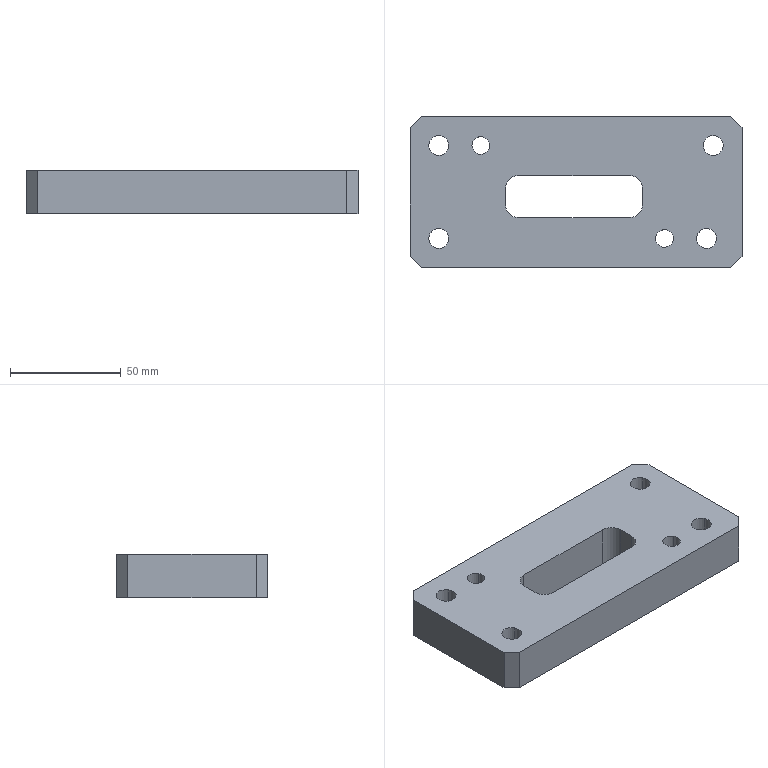Part | CATIA | 1 solid | 42 faces | box 150 x 68 x 19.5 mm | volume 164563 mm3 | cylinder 24 | plane 18 | commonest cylinder face diameters 9 x8 15 x8 8 x4 12 x4
STEP:
#1=CARTESIAN_POINT('',(-305.,34.,20.4));
#2=VERTEX_POINT('',#1);
#3=CARTESIAN_POINT('',(-300.,29.,20.4));
#4=VERTEX_POINT('',#3);
#5=CARTESIAN_POINT('',(-302.5,31.5,20.4));
#6=DIRECTION('',(-0.7071,0.7071,0.));
#7=VECTOR('',#6,1.);
#8=LINE('',#5,#7);
#9=EDGE_CURVE('',#2,#4,#8,.F.);
#10=ORIENTED_EDGE('',*,*,#9,.T.);
#11=CARTESIAN_POINT('',(-300.,29.,0.9));
#12=VERTEX_POINT('',#11);
#13=CARTESIAN_POINT('',(-300.,29.,10.65));
#14=DIRECTION('',(0.,0.,-1.));
#15=VECTOR('',#14,1.);
#16=LINE('',#13,#15);
#17=EDGE_CURVE('',#12,#4,#16,.F.);
#18=ORIENTED_EDGE('',*,*,#17,.F.);
#19=CARTESIAN_POINT('',(-305.,34.,0.9));
#20=VERTEX_POINT('',#19);
#21=CARTESIAN_POINT('',(-302.5,31.5,0.9));
#22=DIRECTION('',(-0.7071,0.7071,0.));
#23=VECTOR('',#22,1.);
#24=LINE('',#21,#23);
#25=EDGE_CURVE('',#12,#20,#24,.T.);
#26=ORIENTED_EDGE('',*,*,#25,.T.);
#27=CARTESIAN_POINT('',(-305.,34.,10.65));
#28=DIRECTION('',(0.,0.,-1.));
#29=VECTOR('',#28,1.);
#30=LINE('',#27,#29);
#31=EDGE_CURVE('',#20,#2,#30,.F.);
#32=ORIENTED_EDGE('',*,*,#31,.T.);
#33=EDGE_LOOP('',(#10,#18,#26,#32));
#34=FACE_OUTER_BOUND('',#33,.T.);
#35=CARTESIAN_POINT('',(-300.,29.,24.3));
#36=DIRECTION('',(0.7071,0.7071,0.));
#37=DIRECTION('',(0.,0.,-1.));
#38=AXIS2_PLACEMENT_3D('',#35,#36,#37);
#39=PLANE('',#38);
#40=ADVANCED_FACE('',(#34),#39,.T.);
#41=CARTESIAN_POINT('',(-445.,34.,0.9));
#42=VERTEX_POINT('',#41);
#43=CARTESIAN_POINT('',(-445.,34.,20.4));
#44=VERTEX_POINT('',#43);
#45=CARTESIAN_POINT('',(-445.,34.,10.65));
#46=DIRECTION('',(0.,0.,1.));
#47=VECTOR('',#46,1.);
#48=LINE('',#45,#47);
#49=EDGE_CURVE('',#42,#44,#48,.T.);
#50=ORIENTED_EDGE('',*,*,#49,.T.);
#51=CARTESIAN_POINT('',(-375.,34.,20.4));
#52=DIRECTION('',(1.,0.,0.));
#53=VECTOR('',#52,1.);
#54=LINE('',#51,#53);
#55=EDGE_CURVE('',#44,#2,#54,.T.);
#56=ORIENTED_EDGE('',*,*,#55,.T.);
#57=ORIENTED_EDGE('',*,*,#31,.F.);
#58=CARTESIAN_POINT('',(-375.,34.,0.9));
#59=DIRECTION('',(1.,0.,0.));
#60=VECTOR('',#59,1.);
#61=LINE('',#58,#60);
#62=EDGE_CURVE('',#20,#42,#61,.F.);
#63=ORIENTED_EDGE('',*,*,#62,.T.);
#64=EDGE_LOOP('',(#50,#56,#57,#63));
#65=FACE_OUTER_BOUND('',#64,.T.);
#66=CARTESIAN_POINT('',(-450.,34.,0.9));
#67=DIRECTION('',(0.,-1.,0.));
#68=DIRECTION('',(1.,0.,0.));
#69=AXIS2_PLACEMENT_3D('',#66,#67,#68);
#70=PLANE('',#69);
#71=ADVANCED_FACE('',(#65),#70,.F.);
#72=CARTESIAN_POINT('',(-450.,29.,20.4));
#73=VERTEX_POINT('',#72);
#74=CARTESIAN_POINT('',(-447.5,31.5,20.4));
#75=DIRECTION('',(0.7071,0.7071,0.));
#76=VECTOR('',#75,1.);
#77=LINE('',#74,#76);
#78=EDGE_CURVE('',#73,#44,#77,.T.);
#79=ORIENTED_EDGE('',*,*,#78,.T.);
#80=ORIENTED_EDGE('',*,*,#49,.F.);
#81=CARTESIAN_POINT('',(-450.,29.,0.9));
#82=VERTEX_POINT('',#81);
#83=CARTESIAN_POINT('',(-447.5,31.5,0.9));
#84=DIRECTION('',(0.7071,0.7071,0.));
#85=VECTOR('',#84,1.);
#86=LINE('',#83,#85);
#87=EDGE_CURVE('',#42,#82,#86,.F.);
#88=ORIENTED_EDGE('',*,*,#87,.T.);
#89=CARTESIAN_POINT('',(-450.,29.,10.65));
#90=DIRECTION('',(0.,0.,1.));
#91=VECTOR('',#90,1.);
#92=LINE('',#89,#91);
#93=EDGE_CURVE('',#82,#73,#92,.T.);
#94=ORIENTED_EDGE('',*,*,#93,.T.);
#95=EDGE_LOOP('',(#79,#80,#88,#94));
#96=FACE_OUTER_BOUND('',#95,.T.);
#97=CARTESIAN_POINT('',(-450.,29.,-3.));
#98=DIRECTION('',(-0.7071,0.7071,0.));
#99=DIRECTION('',(0.,0.,1.));
#100=AXIS2_PLACEMENT_3D('',#97,#98,#99);
#101=PLANE('',#100);
#102=ADVANCED_FACE('',(#96),#101,.T.);
#103=CARTESIAN_POINT('',(-450.,-29.,20.4));
#104=VERTEX_POINT('',#103);
#105=CARTESIAN_POINT('',(-450.,0.,20.4));
#106=DIRECTION('',(0.,-1.,0.));
#107=VECTOR('',#106,1.);
#108=LINE('',#105,#107);
#109=EDGE_CURVE('',#73,#104,#108,.T.);
#110=ORIENTED_EDGE('',*,*,#109,.F.);
#111=ORIENTED_EDGE('',*,*,#93,.F.);
#112=CARTESIAN_POINT('',(-450.,-29.,0.9));
#113=VERTEX_POINT('',#112);
#114=CARTESIAN_POINT('',(-450.,0.,0.9));
#115=DIRECTION('',(0.,-1.,0.));
#116=VECTOR('',#115,1.);
#117=LINE('',#114,#116);
#118=EDGE_CURVE('',#82,#113,#117,.T.);
#119=ORIENTED_EDGE('',*,*,#118,.T.);
#120=CARTESIAN_POINT('',(-450.,-29.,10.65));
#121=DIRECTION('',(0.,0.,-1.));
#122=VECTOR('',#121,1.);
#123=LINE('',#120,#122);
#124=EDGE_CURVE('',#113,#104,#123,.F.);
#125=ORIENTED_EDGE('',*,*,#124,.T.);
#126=EDGE_LOOP('',(#110,#111,#119,#125));
#127=FACE_OUTER_BOUND('',#126,.T.);
#128=CARTESIAN_POINT('',(-450.,34.,0.9));
#129=DIRECTION('',(-1.,0.,0.));
#130=DIRECTION('',(0.,-1.,0.));
#131=AXIS2_PLACEMENT_3D('',#128,#129,#130);
#132=PLANE('',#131);
#133=ADVANCED_FACE('',(#127),#132,.T.);
#134=CARTESIAN_POINT('',(-445.,-34.,20.4));
#135=VERTEX_POINT('',#134);
#136=CARTESIAN_POINT('',(-447.5,-31.5,20.4));
#137=DIRECTION('',(0.7071,-0.7071,0.));
#138=VECTOR('',#137,1.);
#139=LINE('',#136,#138);
#140=EDGE_CURVE('',#135,#104,#139,.F.);
#141=ORIENTED_EDGE('',*,*,#140,.T.);
#142=ORIENTED_EDGE('',*,*,#124,.F.);
#143=CARTESIAN_POINT('',(-445.,-34.,0.9));
#144=VERTEX_POINT('',#143);
#145=CARTESIAN_POINT('',(-447.5,-31.5,0.9));
#146=DIRECTION('',(0.7071,-0.7071,0.));
#147=VECTOR('',#146,1.);
#148=LINE('',#145,#147);
#149=EDGE_CURVE('',#113,#144,#148,.T.);
#150=ORIENTED_EDGE('',*,*,#149,.T.);
#151=CARTESIAN_POINT('',(-445.,-34.,10.65));
#152=DIRECTION('',(0.,0.,-1.));
#153=VECTOR('',#152,1.);
#154=LINE('',#151,#153);
#155=EDGE_CURVE('',#144,#135,#154,.F.);
#156=ORIENTED_EDGE('',*,*,#155,.T.);
#157=EDGE_LOOP('',(#141,#142,#150,#156));
#158=FACE_OUTER_BOUND('',#157,.T.);
#159=CARTESIAN_POINT('',(-450.,-29.,24.3));
#160=DIRECTION('',(-0.7071,-0.7071,0.));
#161=DIRECTION('',(0.,0.,-1.));
#162=AXIS2_PLACEMENT_3D('',#159,#160,#161);
#163=PLANE('',#162);
#164=ADVANCED_FACE('',(#158),#163,.T.);
#165=CARTESIAN_POINT('',(-300.,-29.,0.9));
#166=VERTEX_POINT('',#165);
#167=CARTESIAN_POINT('',(-300.,0.,0.9));
#168=DIRECTION('',(0.,1.,0.));
#169=VECTOR('',#168,1.);
#170=LINE('',#167,#169);
#171=EDGE_CURVE('',#166,#12,#170,.T.);
#172=ORIENTED_EDGE('',*,*,#171,.T.);
#173=ORIENTED_EDGE('',*,*,#17,.T.);
#174=CARTESIAN_POINT('',(-300.,-29.,20.4));
#175=VERTEX_POINT('',#174);
#176=CARTESIAN_POINT('',(-300.,0.,20.4));
#177=DIRECTION('',(0.,1.,0.));
#178=VECTOR('',#177,1.);
#179=LINE('',#176,#178);
#180=EDGE_CURVE('',#175,#4,#179,.T.);
#181=ORIENTED_EDGE('',*,*,#180,.F.);
#182=CARTESIAN_POINT('',(-300.,-29.,10.65));
#183=DIRECTION('',(0.,0.,1.));
#184=VECTOR('',#183,1.);
#185=LINE('',#182,#184);
#186=EDGE_CURVE('',#166,#175,#185,.T.);
#187=ORIENTED_EDGE('',*,*,#186,.F.);
#188=EDGE_LOOP('',(#172,#173,#181,#187));
#189=FACE_OUTER_BOUND('',#188,.T.);
#190=CARTESIAN_POINT('',(-300.,-34.,0.9));
#191=DIRECTION('',(1.,0.,0.));
#192=DIRECTION('',(0.,1.,0.));
#193=AXIS2_PLACEMENT_3D('',#190,#191,#192);
#194=PLANE('',#193);
#195=ADVANCED_FACE('',(#189),#194,.T.);
#196=CARTESIAN_POINT('',(-305.,-34.,0.9));
#197=VERTEX_POINT('',#196);
#198=CARTESIAN_POINT('',(-305.,-34.,20.4));
#199=VERTEX_POINT('',#198);
#200=CARTESIAN_POINT('',(-305.,-34.,10.65));
#201=DIRECTION('',(0.,0.,1.));
#202=VECTOR('',#201,1.);
#203=LINE('',#200,#202);
#204=EDGE_CURVE('',#197,#199,#203,.T.);
#205=ORIENTED_EDGE('',*,*,#204,.T.);
#206=CARTESIAN_POINT('',(-375.,-34.,20.4));
#207=DIRECTION('',(-1.,0.,0.));
#208=VECTOR('',#207,1.);
#209=LINE('',#206,#208);
#210=EDGE_CURVE('',#199,#135,#209,.T.);
#211=ORIENTED_EDGE('',*,*,#210,.T.);
#212=ORIENTED_EDGE('',*,*,#155,.F.);
#213=CARTESIAN_POINT('',(-375.,-34.,0.9));
#214=DIRECTION('',(-1.,0.,0.));
#215=VECTOR('',#214,1.);
#216=LINE('',#213,#215);
#217=EDGE_CURVE('',#144,#197,#216,.F.);
#218=ORIENTED_EDGE('',*,*,#217,.T.);
#219=EDGE_LOOP('',(#205,#211,#212,#218));
#220=FACE_OUTER_BOUND('',#219,.T.);
#221=CARTESIAN_POINT('',(-300.,-34.,0.9));
#222=DIRECTION('',(0.,1.,0.));
#223=DIRECTION('',(-1.,0.,0.));
#224=AXIS2_PLACEMENT_3D('',#221,#222,#223);
#225=PLANE('',#224);
#226=ADVANCED_FACE('',(#220),#225,.F.);
#227=CARTESIAN_POINT('',(-302.5,-31.5,20.4));
#228=DIRECTION('',(-0.7071,-0.7071,0.));
#229=VECTOR('',#228,1.);
#230=LINE('',#227,#229);
#231=EDGE_CURVE('',#175,#199,#230,.T.);
#232=ORIENTED_EDGE('',*,*,#231,.T.);
#233=ORIENTED_EDGE('',*,*,#204,.F.);
#234=CARTESIAN_POINT('',(-302.5,-31.5,0.9));
#235=DIRECTION('',(-0.7071,-0.7071,0.));
#236=VECTOR('',#235,1.);
#237=LINE('',#234,#236);
#238=EDGE_CURVE('',#197,#166,#237,.F.);
#239=ORIENTED_EDGE('',*,*,#238,.T.);
#240=ORIENTED_EDGE('',*,*,#186,.T.);
#241=EDGE_LOOP('',(#232,#233,#239,#240));
#242=FACE_OUTER_BOUND('',#241,.T.);
#243=CARTESIAN_POINT('',(-300.,-29.,-3.));
#244=DIRECTION('',(0.7071,-0.7071,0.));
#245=DIRECTION('',(0.,0.,1.));
#246=AXIS2_PLACEMENT_3D('',#243,#244,#245);
#247=PLANE('',#246);
#248=ADVANCED_FACE('',(#242),#247,.T.);
#249=CARTESIAN_POINT('',(-350.9,-11.6,20.4));
#250=VERTEX_POINT('',#249);
#251=CARTESIAN_POINT('',(-344.9,-5.6,20.4));
#252=VERTEX_POINT('',#251);
#253=CARTESIAN_POINT('',(-350.9,-5.6,20.4));
#254=DIRECTION('',(0.,0.,-1.));
#255=AXIS2_PLACEMENT_3D('',#253,#254,$);
#256=CIRCLE('',#255,6.);
#257=EDGE_CURVE('',#250,#252,#256,.F.);
#258=ORIENTED_EDGE('',*,*,#257,.T.);
#259=CARTESIAN_POINT('',(-344.9,-5.6,0.9));
#260=VERTEX_POINT('',#259);
#261=CARTESIAN_POINT('',(-344.9,-5.6,39.4));
#262=DIRECTION('',(0.,0.,-1.));
#263=VECTOR('',#262,1.);
#264=LINE('',#261,#263);
#265=EDGE_CURVE('',#252,#260,#264,.T.);
#266=ORIENTED_EDGE('',*,*,#265,.T.);
#267=CARTESIAN_POINT('',(-350.9,-11.6,0.9));
#268=VERTEX_POINT('',#267);
#269=CARTESIAN_POINT('',(-350.9,-5.6,0.9));
#270=DIRECTION('',(0.,0.,-1.));
#271=AXIS2_PLACEMENT_3D('',#269,#270,$);
#272=CIRCLE('',#271,6.);
#273=EDGE_CURVE('',#268,#260,#272,.F.);
#274=ORIENTED_EDGE('',*,*,#273,.F.);
#275=CARTESIAN_POINT('',(-350.9,-11.6,39.4));
#276=DIRECTION('',(0.,0.,-1.));
#277=VECTOR('',#276,1.);
#278=LINE('',#275,#277);
#279=EDGE_CURVE('',#250,#268,#278,.T.);
#280=ORIENTED_EDGE('',*,*,#279,.F.);
#281=EDGE_LOOP('',(#258,#266,#274,#280));
#282=FACE_OUTER_BOUND('',#281,.T.);
#283=CARTESIAN_POINT('',(-350.9,-5.6,39.4));
#284=DIRECTION('',(0.,0.,-1.));
#285=DIRECTION('',(1.,0.,0.));
#286=AXIS2_PLACEMENT_3D('',#283,#284,#285);
#287=CYLINDRICAL_SURFACE('',#286,6.);
#288=ADVANCED_FACE('',(#282),#287,.F.);
#289=ORIENTED_EDGE('',*,*,#279,.T.);
#290=CARTESIAN_POINT('',(-400.9,-11.6,0.9));
#291=VERTEX_POINT('',#290);
#292=CARTESIAN_POINT('',(-375.9,-11.6,0.9));
#293=DIRECTION('',(1.,0.,0.));
#294=VECTOR('',#293,1.);
#295=LINE('',#292,#294);
#296=EDGE_CURVE('',#291,#268,#295,.T.);
#297=ORIENTED_EDGE('',*,*,#296,.F.);
#298=CARTESIAN_POINT('',(-400.9,-11.6,20.4));
#299=VERTEX_POINT('',#298);
#300=CARTESIAN_POINT('',(-400.9,-11.6,39.4));
#301=DIRECTION('',(0.,0.,-1.));
#302=VECTOR('',#301,1.);
#303=LINE('',#300,#302);
#304=EDGE_CURVE('',#299,#291,#303,.T.);
#305=ORIENTED_EDGE('',*,*,#304,.F.);
#306=CARTESIAN_POINT('',(-375.9,-11.6,20.4));
#307=DIRECTION('',(1.,0.,0.));
#308=VECTOR('',#307,1.);
#309=LINE('',#306,#308);
#310=EDGE_CURVE('',#299,#250,#309,.T.);
#311=ORIENTED_EDGE('',*,*,#310,.T.);
#312=EDGE_LOOP('',(#289,#297,#305,#311));
#313=FACE_OUTER_BOUND('',#312,.T.);
#314=CARTESIAN_POINT('',(-401.9,-11.6,17.9));
#315=DIRECTION('',(0.,1.,0.));
#316=DIRECTION('',(1.,0.,0.));
#317=AXIS2_PLACEMENT_3D('',#314,#315,#316);
#318=PLANE('',#317);
#319=ADVANCED_FACE('',(#313),#318,.T.);
#320=CARTESIAN_POINT('',(-344.9,1.4,20.4));
#321=VERTEX_POINT('',#320);
#322=CARTESIAN_POINT('',(-344.9,-2.1,20.4));
#323=DIRECTION('',(0.,-1.,0.));
#324=VECTOR('',#323,1.);
#325=LINE('',#322,#324);
#326=EDGE_CURVE('',#321,#252,#325,.T.);
#327=ORIENTED_EDGE('',*,*,#326,.F.);
#328=CARTESIAN_POINT('',(-344.9,1.4,0.9));
#329=VERTEX_POINT('',#328);
#330=CARTESIAN_POINT('',(-344.9,1.4,39.4));
#331=DIRECTION('',(0.,0.,-1.));
#332=VECTOR('',#331,1.);
#333=LINE('',#330,#332);
#334=EDGE_CURVE('',#321,#329,#333,.T.);
#335=ORIENTED_EDGE('',*,*,#334,.T.);
#336=CARTESIAN_POINT('',(-344.9,-2.1,0.9));
#337=DIRECTION('',(0.,-1.,0.));
#338=VECTOR('',#337,1.);
#339=LINE('',#336,#338);
#340=EDGE_CURVE('',#260,#329,#339,.F.);
#341=ORIENTED_EDGE('',*,*,#340,.F.);
#342=ORIENTED_EDGE('',*,*,#265,.F.);
#343=EDGE_LOOP('',(#327,#335,#341,#342));
#344=FACE_OUTER_BOUND('',#343,.T.);
#345=CARTESIAN_POINT('',(-344.9,2.4,17.9));
#346=DIRECTION('',(1.,0.,0.));
#347=DIRECTION('',(0.,-1.,0.));
#348=AXIS2_PLACEMENT_3D('',#345,#346,#347);
#349=PLANE('',#348);
#350=ADVANCED_FACE('',(#344),#349,.F.);
#351=CARTESIAN_POINT('',(-406.9,-5.6,20.4));
#352=VERTEX_POINT('',#351);
#353=CARTESIAN_POINT('',(-400.9,-5.6,20.4));
#354=DIRECTION('',(0.,0.,-1.));
#355=AXIS2_PLACEMENT_3D('',#353,#354,$);
#356=CIRCLE('',#355,6.);
#357=EDGE_CURVE('',#352,#299,#356,.F.);
#358=ORIENTED_EDGE('',*,*,#357,.T.);
#359=ORIENTED_EDGE('',*,*,#304,.T.);
#360=CARTESIAN_POINT('',(-406.9,-5.6,0.9));
#361=VERTEX_POINT('',#360);
#362=CARTESIAN_POINT('',(-400.9,-5.6,0.9));
#363=DIRECTION('',(0.,0.,-1.));
#364=AXIS2_PLACEMENT_3D('',#362,#363,$);
#365=CIRCLE('',#364,6.);
#366=EDGE_CURVE('',#361,#291,#365,.F.);
#367=ORIENTED_EDGE('',*,*,#366,.F.);
#368=CARTESIAN_POINT('',(-406.9,-5.6,39.4));
#369=DIRECTION('',(0.,0.,-1.));
#370=VECTOR('',#369,1.);
#371=LINE('',#368,#370);
#372=EDGE_CURVE('',#352,#361,#371,.T.);
#373=ORIENTED_EDGE('',*,*,#372,.F.);
#374=EDGE_LOOP('',(#358,#359,#367,#373));
#375=FACE_OUTER_BOUND('',#374,.T.);
#376=CARTESIAN_POINT('',(-400.9,-5.6,39.4));
#377=DIRECTION('',(0.,0.,-1.));
#378=DIRECTION('',(0.,-1.,0.));
#379=AXIS2_PLACEMENT_3D('',#376,#377,#378);
#380=CYLINDRICAL_SURFACE('',#379,6.);
#381=ADVANCED_FACE('',(#375),#380,.F.);
#382=CARTESIAN_POINT('',(-350.9,7.4,20.4));
#383=VERTEX_POINT('',#382);
#384=CARTESIAN_POINT('',(-350.9,1.4,20.4));
#385=DIRECTION('',(0.,0.,-1.));
#386=AXIS2_PLACEMENT_3D('',#384,#385,$);
#387=CIRCLE('',#386,6.);
#388=EDGE_CURVE('',#321,#383,#387,.F.);
#389=ORIENTED_EDGE('',*,*,#388,.T.);
#390=CARTESIAN_POINT('',(-350.9,7.4,0.9));
#391=VERTEX_POINT('',#390);
#392=CARTESIAN_POINT('',(-350.9,7.4,39.4));
#393=DIRECTION('',(0.,0.,-1.));
#394=VECTOR('',#393,1.);
#395=LINE('',#392,#394);
#396=EDGE_CURVE('',#383,#391,#395,.T.);
#397=ORIENTED_EDGE('',*,*,#396,.T.);
#398=CARTESIAN_POINT('',(-350.9,1.4,0.9));
#399=DIRECTION('',(0.,0.,-1.));
#400=AXIS2_PLACEMENT_3D('',#398,#399,$);
#401=CIRCLE('',#400,6.);
#402=EDGE_CURVE('',#329,#391,#401,.F.);
#403=ORIENTED_EDGE('',*,*,#402,.F.);
#404=ORIENTED_EDGE('',*,*,#334,.F.);
#405=EDGE_LOOP('',(#389,#397,#403,#404));
#406=FACE_OUTER_BOUND('',#405,.T.);
#407=CARTESIAN_POINT('',(-350.9,1.4,39.4));
#408=DIRECTION('',(0.,0.,-1.));
#409=DIRECTION('',(0.,1.,0.));
#410=AXIS2_PLACEMENT_3D('',#407,#408,#409);
#411=CYLINDRICAL_SURFACE('',#410,6.);
#412=ADVANCED_FACE('',(#406),#411,.F.);
#413=CARTESIAN_POINT('',(-406.9,1.4,20.4));
#414=VERTEX_POINT('',#413);
#415=CARTESIAN_POINT('',(-406.9,-2.1,20.4));
#416=DIRECTION('',(0.,1.,0.));
#417=VECTOR('',#416,1.);
#418=LINE('',#415,#417);
#419=EDGE_CURVE('',#352,#414,#418,.T.);
#420=ORIENTED_EDGE('',*,*,#419,.F.);
#421=ORIENTED_EDGE('',*,*,#372,.T.);
#422=CARTESIAN_POINT('',(-406.9,1.4,0.9));
#423=VERTEX_POINT('',#422);
#424=CARTESIAN_POINT('',(-406.9,-2.1,0.9));
#425=DIRECTION('',(0.,1.,0.));
#426=VECTOR('',#425,1.);
#427=LINE('',#424,#426);
#428=EDGE_CURVE('',#361,#423,#427,.T.);
#429=ORIENTED_EDGE('',*,*,#428,.T.);
#430=CARTESIAN_POINT('',(-406.9,1.4,39.4));
#431=DIRECTION('',(0.,0.,-1.));
#432=VECTOR('',#431,1.);
#433=LINE('',#430,#432);
#434=EDGE_CURVE('',#414,#423,#433,.T.);
#435=ORIENTED_EDGE('',*,*,#434,.F.);
#436=EDGE_LOOP('',(#420,#421,#429,#435));
#437=FACE_OUTER_BOUND('',#436,.T.);
#438=CARTESIAN_POINT('',(-406.9,-6.6,17.9));
#439=DIRECTION('',(-1.,0.,0.));
#440=DIRECTION('',(0.,1.,0.));
#441=AXIS2_PLACEMENT_3D('',#438,#439,#440);
#442=PLANE('',#441);
#443=ADVANCED_FACE('',(#437),#442,.F.);
#444=CARTESIAN_POINT('',(-400.9,7.4,20.4));
#445=VERTEX_POINT('',#444);
#446=CARTESIAN_POINT('',(-400.9,7.4,0.9));
#447=VERTEX_POINT('',#446);
#448=CARTESIAN_POINT('',(-400.9,7.4,39.4));
#449=DIRECTION('',(0.,0.,-1.));
#450=VECTOR('',#449,1.);
#451=LINE('',#448,#450);
#452=EDGE_CURVE('',#445,#447,#451,.T.);
#453=ORIENTED_EDGE('',*,*,#452,.T.);
#454=CARTESIAN_POINT('',(-375.9,7.4,0.9));
#455=DIRECTION('',(-1.,0.,0.));
#456=VECTOR('',#455,1.);
#457=LINE('',#454,#456);
#458=EDGE_CURVE('',#447,#391,#457,.F.);
#459=ORIENTED_EDGE('',*,*,#458,.T.);
#460=ORIENTED_EDGE('',*,*,#396,.F.);
#461=CARTESIAN_POINT('',(-375.9,7.4,20.4));
#462=DIRECTION('',(-1.,0.,0.));
#463=VECTOR('',#462,1.);
#464=LINE('',#461,#463);
#465=EDGE_CURVE('',#383,#445,#464,.T.);
#466=ORIENTED_EDGE('',*,*,#465,.T.);
#467=EDGE_LOOP('',(#453,#459,#460,#466));
#468=FACE_OUTER_BOUND('',#467,.T.);
#469=CARTESIAN_POINT('',(-349.9,7.4,17.9));
#470=DIRECTION('',(0.,-1.,0.));
#471=DIRECTION('',(-1.,0.,0.));
#472=AXIS2_PLACEMENT_3D('',#469,#470,#471);
#473=PLANE('',#472);
#474=ADVANCED_FACE('',(#468),#473,.T.);
#475=CARTESIAN_POINT('',(-400.9,1.4,20.4));
#476=DIRECTION('',(0.,0.,-1.));
#477=AXIS2_PLACEMENT_3D('',#475,#476,$);
#478=CIRCLE('',#477,6.);
#479=EDGE_CURVE('',#445,#414,#478,.F.);
#480=ORIENTED_EDGE('',*,*,#479,.T.);
#481=ORIENTED_EDGE('',*,*,#434,.T.);
#482=CARTESIAN_POINT('',(-400.9,1.4,0.9));
#483=DIRECTION('',(0.,0.,-1.));
#484=AXIS2_PLACEMENT_3D('',#482,#483,$);
#485=CIRCLE('',#484,6.);
#486=EDGE_CURVE('',#447,#423,#485,.F.);
#487=ORIENTED_EDGE('',*,*,#486,.F.);
#488=ORIENTED_EDGE('',*,*,#452,.F.);
#489=EDGE_LOOP('',(#480,#481,#487,#488));
#490=FACE_OUTER_BOUND('',#489,.T.);
#491=CARTESIAN_POINT('',(-400.9,1.4,39.4));
#492=DIRECTION('',(0.,0.,-1.));
#493=DIRECTION('',(-1.,0.,0.));
#494=AXIS2_PLACEMENT_3D('',#491,#492,#493);
#495=CYLINDRICAL_SURFACE('',#494,6.);
#496=ADVANCED_FACE('',(#490),#495,.F.);
#497=ORIENTED_EDGE('',*,*,#238,.F.);
#498=ORIENTED_EDGE('',*,*,#217,.F.);
#499=ORIENTED_EDGE('',*,*,#149,.F.);
#500=ORIENTED_EDGE('',*,*,#118,.F.);
#501=ORIENTED_EDGE('',*,*,#87,.F.);
#502=ORIENTED_EDGE('',*,*,#62,.F.);
#503=ORIENTED_EDGE('',*,*,#25,.F.);
#504=ORIENTED_EDGE('',*,*,#171,.F.);
#505=EDGE_LOOP('',(#497,#498,#499,#500,#501,#502,#503,#504));
#506=FACE_OUTER_BOUND('',#505,.T.);
#507=ORIENTED_EDGE('',*,*,#273,.T.);
#508=ORIENTED_EDGE('',*,*,#340,.T.);
#509=ORIENTED_EDGE('',*,*,#402,.T.);
#510=ORIENTED_EDGE('',*,*,#458,.F.);
#511=ORIENTED_EDGE('',*,*,#486,.T.);
#512=ORIENTED_EDGE('',*,*,#428,.F.);
#513=ORIENTED_EDGE('',*,*,#366,.T.);
#514=ORIENTED_EDGE('',*,*,#296,.T.);
#515=EDGE_LOOP('',(#507,#508,#509,#510,#511,#512,#513,#514));
#516=FACE_BOUND('',#515,.T.);
#517=CARTESIAN_POINT('',(-306.418,24.596,0.9));
#518=VERTEX_POINT('',#517);
#519=CARTESIAN_POINT('',(-319.582,17.404,0.9));
#520=VERTEX_POINT('',#519);
#521=CARTESIAN_POINT('',(-313.,21.,0.9));
#522=DIRECTION('',(0.,0.,1.));
#523=AXIS2_PLACEMENT_3D('',#521,#522,$);
#524=CIRCLE('',#523,7.5);
#525=EDGE_CURVE('',#518,#520,#524,.T.);
#526=ORIENTED_EDGE('',*,*,#525,.T.);
#527=CARTESIAN_POINT('',(-313.,21.,0.9));
#528=DIRECTION('',(0.,0.,1.));
#529=AXIS2_PLACEMENT_3D('',#527,#528,$);
#530=CIRCLE('',#529,7.5);
#531=EDGE_CURVE('',#520,#518,#530,.T.);
#532=ORIENTED_EDGE('',*,*,#531,.T.);
#533=EDGE_LOOP('',(#526,#532));
#534=FACE_BOUND('',#533,.T.);
#535=CARTESIAN_POINT('',(-430.418,24.596,0.9));
#536=VERTEX_POINT('',#535);
#537=CARTESIAN_POINT('',(-443.582,17.404,0.9));
#538=VERTEX_POINT('',#537);
#539=CARTESIAN_POINT('',(-437.,21.,0.9));
#540=DIRECTION('',(0.,0.,1.));
#541=AXIS2_PLACEMENT_3D('',#539,#540,$);
#542=CIRCLE('',#541,7.5);
#543=EDGE_CURVE('',#536,#538,#542,.T.);
#544=ORIENTED_EDGE('',*,*,#543,.T.);
#545=CARTESIAN_POINT('',(-437.,21.,0.9));
#546=DIRECTION('',(0.,0.,1.));
#547=AXIS2_PLACEMENT_3D('',#545,#546,$);
#548=CIRCLE('',#547,7.5);
#549=EDGE_CURVE('',#538,#536,#548,.T.);
#550=ORIENTED_EDGE('',*,*,#549,.T.);
#551=EDGE_LOOP('',(#544,#550));
#552=FACE_BOUND('',#551,.T.);
#553=CARTESIAN_POINT('',(-430.418,-17.404,0.9));
#554=VERTEX_POINT('',#553);
#555=CARTESIAN_POINT('',(-443.582,-24.596,0.9));
#556=VERTEX_POINT('',#555);
#557=CARTESIAN_POINT('',(-437.,-21.,0.9));
#558=DIRECTION('',(0.,0.,1.));
#559=AXIS2_PLACEMENT_3D('',#557,#558,$);
#560=CIRCLE('',#559,7.5);
#561=EDGE_CURVE('',#554,#556,#560,.T.);
#562=ORIENTED_EDGE('',*,*,#561,.T.);
#563=CARTESIAN_POINT('',(-437.,-21.,0.9));
#564=DIRECTION('',(0.,0.,1.));
#565=AXIS2_PLACEMENT_3D('',#563,#564,$);
#566=CIRCLE('',#565,7.5);
#567=EDGE_CURVE('',#556,#554,#566,.T.);
#568=ORIENTED_EDGE('',*,*,#567,.T.);
#569=EDGE_LOOP('',(#562,#568));
#570=FACE_BOUND('',#569,.T.);
#571=CARTESIAN_POINT('',(-309.418,-17.404,0.9));
#572=VERTEX_POINT('',#571);
#573=CARTESIAN_POINT('',(-322.582,-24.596,0.9));
#574=VERTEX_POINT('',#573);
#575=CARTESIAN_POINT('',(-316.,-21.,0.9));
#576=DIRECTION('',(0.,0.,1.));
#577=AXIS2_PLACEMENT_3D('',#575,#576,$);
#578=CIRCLE('',#577,7.5);
#579=EDGE_CURVE('',#572,#574,#578,.T.);
#580=ORIENTED_EDGE('',*,*,#579,.T.);
#581=CARTESIAN_POINT('',(-316.,-21.,0.9));
#582=DIRECTION('',(0.,0.,1.));
#583=AXIS2_PLACEMENT_3D('',#581,#582,$);
#584=CIRCLE('',#583,7.5);
#585=EDGE_CURVE('',#574,#572,#584,.T.);
#586=ORIENTED_EDGE('',*,*,#585,.T.);
#587=EDGE_LOOP('',(#580,#586));
#588=FACE_BOUND('',#587,.T.);
#589=CARTESIAN_POINT('',(-338.51,-22.918,0.9));
#590=VERTEX_POINT('',#589);
#591=CARTESIAN_POINT('',(-331.49,-19.082,0.9));
#592=VERTEX_POINT('',#591);
#593=CARTESIAN_POINT('',(-335.,-21.,0.9));
#594=DIRECTION('',(0.,0.,1.));
#595=AXIS2_PLACEMENT_3D('',#593,#594,$);
#596=CIRCLE('',#595,4.);
#597=EDGE_CURVE('',#590,#592,#596,.T.);
#598=ORIENTED_EDGE('',*,*,#597,.T.);
#599=CARTESIAN_POINT('',(-335.,-21.,0.9));
#600=DIRECTION('',(0.,0.,1.));
#601=AXIS2_PLACEMENT_3D('',#599,#600,$);
#602=CIRCLE('',#601,4.);
#603=EDGE_CURVE('',#592,#590,#602,.T.);
#604=ORIENTED_EDGE('',*,*,#603,.T.);
#605=EDGE_LOOP('',(#598,#604));
#606=FACE_BOUND('',#605,.T.);
#607=CARTESIAN_POINT('',(-421.51,19.082,0.9));
#608=VERTEX_POINT('',#607);
#609=CARTESIAN_POINT('',(-414.49,22.918,0.9));
#610=VERTEX_POINT('',#609);
#611=CARTESIAN_POINT('',(-418.,21.,0.9));
#612=DIRECTION('',(0.,0.,1.));
#613=AXIS2_PLACEMENT_3D('',#611,#612,$);
#614=CIRCLE('',#613,4.);
#615=EDGE_CURVE('',#608,#610,#614,.T.);
#616=ORIENTED_EDGE('',*,*,#615,.T.);
#617=CARTESIAN_POINT('',(-418.,21.,0.9));
#618=DIRECTION('',(0.,0.,1.));
#619=AXIS2_PLACEMENT_3D('',#617,#618,$);
#620=CIRCLE('',#619,4.);
#621=EDGE_CURVE('',#610,#608,#620,.T.);
#622=ORIENTED_EDGE('',*,*,#621,.T.);
#623=EDGE_LOOP('',(#616,#622));
#624=FACE_BOUND('',#623,.T.);
#625=CARTESIAN_POINT('',(0.,0.,0.9));
#626=DIRECTION('',(0.,0.,1.));
#627=DIRECTION('',(1.,0.,0.));
#628=AXIS2_PLACEMENT_3D('',#625,#626,#627);
#629=PLANE('',#628);
#630=ADVANCED_FACE('',(#506,#516,#534,#552,#570,#588,#606,#624),#629,.F.);
#631=ORIENTED_EDGE('',*,*,#180,.T.);
#632=ORIENTED_EDGE('',*,*,#9,.F.);
#633=ORIENTED_EDGE('',*,*,#55,.F.);
#634=ORIENTED_EDGE('',*,*,#78,.F.);
#635=ORIENTED_EDGE('',*,*,#109,.T.);
#636=ORIENTED_EDGE('',*,*,#140,.F.);
#637=ORIENTED_EDGE('',*,*,#210,.F.);
#638=ORIENTED_EDGE('',*,*,#231,.F.);
#639=EDGE_LOOP('',(#631,#632,#633,#634,#635,#636,#637,#638));
#640=FACE_OUTER_BOUND('',#639,.T.);
#641=ORIENTED_EDGE('',*,*,#310,.F.);
#642=ORIENTED_EDGE('',*,*,#357,.F.);
#643=ORIENTED_EDGE('',*,*,#419,.T.);
#644=ORIENTED_EDGE('',*,*,#479,.F.);
#645=ORIENTED_EDGE('',*,*,#465,.F.);
#646=ORIENTED_EDGE('',*,*,#388,.F.);
#647=ORIENTED_EDGE('',*,*,#326,.T.);
#648=ORIENTED_EDGE('',*,*,#257,.F.);
#649=EDGE_LOOP('',(#641,#642,#643,#644,#645,#646,#647,#648));
#650=FACE_BOUND('',#649,.T.);
#651=CARTESIAN_POINT('',(-316.949,18.843,20.4));
#652=VERTEX_POINT('',#651);
#653=CARTESIAN_POINT('',(-309.051,23.157,20.4));
#654=VERTEX_POINT('',#653);
#655=CARTESIAN_POINT('',(-313.,21.,20.4));
#656=DIRECTION('',(0.,0.,1.));
#657=AXIS2_PLACEMENT_3D('',#655,#656,$);
#658=CIRCLE('',#657,4.5);
#659=EDGE_CURVE('',#652,#654,#658,.T.);
#660=ORIENTED_EDGE('',*,*,#659,.F.);
#661=CARTESIAN_POINT('',(-313.,21.,20.4));
#662=DIRECTION('',(0.,0.,1.));
#663=AXIS2_PLACEMENT_3D('',#661,#662,$);
#664=CIRCLE('',#663,4.5);
#665=EDGE_CURVE('',#654,#652,#664,.T.);
#666=ORIENTED_EDGE('',*,*,#665,.F.);
#667=EDGE_LOOP('',(#660,#666));
#668=FACE_BOUND('',#667,.T.);
#669=CARTESIAN_POINT('',(-440.949,18.843,20.4));
#670=VERTEX_POINT('',#669);
#671=CARTESIAN_POINT('',(-433.051,23.157,20.4));
#672=VERTEX_POINT('',#671);
#673=CARTESIAN_POINT('',(-437.,21.,20.4));
#674=DIRECTION('',(0.,0.,1.));
#675=AXIS2_PLACEMENT_3D('',#673,#674,$);
#676=CIRCLE('',#675,4.5);
#677=EDGE_CURVE('',#670,#672,#676,.T.);
#678=ORIENTED_EDGE('',*,*,#677,.F.);
#679=CARTESIAN_POINT('',(-437.,21.,20.4));
#680=DIRECTION('',(0.,0.,1.));
#681=AXIS2_PLACEMENT_3D('',#679,#680,$);
#682=CIRCLE('',#681,4.5);
#683=EDGE_CURVE('',#672,#670,#682,.T.);
#684=ORIENTED_EDGE('',*,*,#683,.F.);
#685=EDGE_LOOP('',(#678,#684));
#686=FACE_BOUND('',#685,.T.);
#687=CARTESIAN_POINT('',(-440.949,-23.157,20.4));
#688=VERTEX_POINT('',#687);
#689=CARTESIAN_POINT('',(-433.051,-18.843,20.4));
#690=VERTEX_POINT('',#689);
#691=CARTESIAN_POINT('',(-437.,-21.,20.4));
#692=DIRECTION('',(0.,0.,1.));
#693=AXIS2_PLACEMENT_3D('',#691,#692,$);
#694=CIRCLE('',#693,4.5);
#695=EDGE_CURVE('',#688,#690,#694,.T.);
#696=ORIENTED_EDGE('',*,*,#695,.F.);
#697=CARTESIAN_POINT('',(-437.,-21.,20.4));
#698=DIRECTION('',(0.,0.,1.));
#699=AXIS2_PLACEMENT_3D('',#697,#698,$);
#700=CIRCLE('',#699,4.5);
#701=EDGE_CURVE('',#690,#688,#700,.T.);
#702=ORIENTED_EDGE('',*,*,#701,.F.);
#703=EDGE_LOOP('',(#696,#702));
#704=FACE_BOUND('',#703,.T.);
#705=CARTESIAN_POINT('',(-319.949,-23.157,20.4));
#706=VERTEX_POINT('',#705);
#707=CARTESIAN_POINT('',(-312.051,-18.843,20.4));
#708=VERTEX_POINT('',#707);
#709=CARTESIAN_POINT('',(-316.,-21.,20.4));
#710=DIRECTION('',(0.,0.,1.));
#711=AXIS2_PLACEMENT_3D('',#709,#710,$);
#712=CIRCLE('',#711,4.5);
#713=EDGE_CURVE('',#706,#708,#712,.T.);
#714=ORIENTED_EDGE('',*,*,#713,.F.);
#715=CARTESIAN_POINT('',(-316.,-21.,20.4));
#716=DIRECTION('',(0.,0.,1.));
#717=AXIS2_PLACEMENT_3D('',#715,#716,$);
#718=CIRCLE('',#717,4.5);
#719=EDGE_CURVE('',#708,#706,#718,.T.);
#720=ORIENTED_EDGE('',*,*,#719,.F.);
#721=EDGE_LOOP('',(#714,#720));
#722=FACE_BOUND('',#721,.T.);
#723=CARTESIAN_POINT('',(-338.51,-22.918,20.4));
#724=VERTEX_POINT('',#723);
#725=CARTESIAN_POINT('',(-331.49,-19.082,20.4));
#726=VERTEX_POINT('',#725);
#727=CARTESIAN_POINT('',(-335.,-21.,20.4));
#728=DIRECTION('',(0.,0.,1.));
#729=AXIS2_PLACEMENT_3D('',#727,#728,$);
#730=CIRCLE('',#729,4.);
#731=EDGE_CURVE('',#724,#726,#730,.T.);
#732=ORIENTED_EDGE('',*,*,#731,.F.);
#733=CARTESIAN_POINT('',(-335.,-21.,20.4));
#734=DIRECTION('',(0.,0.,1.));
#735=AXIS2_PLACEMENT_3D('',#733,#734,$);
#736=CIRCLE('',#735,4.);
#737=EDGE_CURVE('',#726,#724,#736,.T.);
#738=ORIENTED_EDGE('',*,*,#737,.F.);
#739=EDGE_LOOP('',(#732,#738));
#740=FACE_BOUND('',#739,.T.);
#741=CARTESIAN_POINT('',(-421.51,19.082,20.4));
#742=VERTEX_POINT('',#741);
#743=CARTESIAN_POINT('',(-414.49,22.918,20.4));
#744=VERTEX_POINT('',#743);
#745=CARTESIAN_POINT('',(-418.,21.,20.4));
#746=DIRECTION('',(0.,0.,1.));
#747=AXIS2_PLACEMENT_3D('',#745,#746,$);
#748=CIRCLE('',#747,4.);
#749=EDGE_CURVE('',#742,#744,#748,.T.);
#750=ORIENTED_EDGE('',*,*,#749,.F.);
#751=CARTESIAN_POINT('',(-418.,21.,20.4));
#752=DIRECTION('',(0.,0.,1.));
#753=AXIS2_PLACEMENT_3D('',#751,#752,$);
#754=CIRCLE('',#753,4.);
#755=EDGE_CURVE('',#744,#742,#754,.T.);
#756=ORIENTED_EDGE('',*,*,#755,.F.);
#757=EDGE_LOOP('',(#750,#756));
#758=FACE_BOUND('',#757,.T.);
#759=CARTESIAN_POINT('',(0.,0.,20.4));
#760=DIRECTION('',(0.,0.,1.));
#761=DIRECTION('',(1.,0.,0.));
#762=AXIS2_PLACEMENT_3D('',#759,#760,#761);
#763=PLANE('',#762);
#764=ADVANCED_FACE('',(#640,#650,#668,#686,#704,#722,#740,#758),#763,.T.);
#765=CARTESIAN_POINT('',(-309.418,-17.404,9.9));
#766=VERTEX_POINT('',#765);
#767=CARTESIAN_POINT('',(-322.582,-24.596,9.9));
#768=VERTEX_POINT('',#767);
#769=CARTESIAN_POINT('',(-316.,-21.,9.9));
#770=DIRECTION('',(0.,0.,1.));
#771=AXIS2_PLACEMENT_3D('',#769,#770,$);
#772=CIRCLE('',#771,7.5);
#773=EDGE_CURVE('',#766,#768,#772,.T.);
#774=ORIENTED_EDGE('',*,*,#773,.F.);
#775=CARTESIAN_POINT('',(-316.,-21.,9.9));
#776=DIRECTION('',(0.,0.,1.));
#777=AXIS2_PLACEMENT_3D('',#775,#776,$);
#778=CIRCLE('',#777,7.5);
#779=EDGE_CURVE('',#768,#766,#778,.T.);
#780=ORIENTED_EDGE('',*,*,#779,.F.);
#781=EDGE_LOOP('',(#774,#780));
#782=FACE_OUTER_BOUND('',#781,.T.);
#783=CARTESIAN_POINT('',(-319.949,-23.157,9.9));
#784=VERTEX_POINT('',#783);
#785=CARTESIAN_POINT('',(-312.051,-18.843,9.9));
#786=VERTEX_POINT('',#785);
#787=CARTESIAN_POINT('',(-316.,-21.,9.9));
#788=DIRECTION('',(0.,0.,1.));
#789=AXIS2_PLACEMENT_3D('',#787,#788,$);
#790=CIRCLE('',#789,4.5);
#791=EDGE_CURVE('',#784,#786,#790,.T.);
#792=ORIENTED_EDGE('',*,*,#791,.T.);
#793=CARTESIAN_POINT('',(-316.,-21.,9.9));
#794=DIRECTION('',(0.,0.,1.));
#795=AXIS2_PLACEMENT_3D('',#793,#794,$);
#796=CIRCLE('',#795,4.5);
#797=EDGE_CURVE('',#786,#784,#796,.T.);
#798=ORIENTED_EDGE('',*,*,#797,.T.);
#799=EDGE_LOOP('',(#792,#798));
#800=FACE_BOUND('',#799,.T.);
#801=CARTESIAN_POINT('',(-308.5,21.,9.9));
#802=DIRECTION('',(0.,0.,1.));
#803=DIRECTION('',(1.,0.,0.));
#804=AXIS2_PLACEMENT_3D('',#801,#802,#803);
#805=PLANE('',#804);
#806=ADVANCED_FACE('',(#782,#800),#805,.F.);
#807=ORIENTED_EDGE('',*,*,#585,.F.);
#808=CARTESIAN_POINT('',(-322.582,-24.596,5.245));
#809=DIRECTION('',(0.,0.,1.));
#810=VECTOR('',#809,1.);
#811=LINE('',#808,#810);
#812=EDGE_CURVE('',#768,#574,#811,.F.);
#813=ORIENTED_EDGE('',*,*,#812,.F.);
#814=ORIENTED_EDGE('',*,*,#779,.T.);
#815=CARTESIAN_POINT('',(-309.418,-17.404,5.245));
#816=DIRECTION('',(0.,0.,1.));
#817=VECTOR('',#816,1.);
#818=LINE('',#815,#817);
#819=EDGE_CURVE('',#766,#572,#818,.F.);
#820=ORIENTED_EDGE('',*,*,#819,.T.);
#821=EDGE_LOOP('',(#807,#813,#814,#820));
#822=FACE_OUTER_BOUND('',#821,.T.);
#823=CARTESIAN_POINT('',(-316.,-21.,1.));
#824=DIRECTION('',(0.,0.,1.));
#825=DIRECTION('',(0.8776,0.4794,0.));
#826=AXIS2_PLACEMENT_3D('',#823,#824,#825);
#827=CYLINDRICAL_SURFACE('',#826,7.5);
#828=ADVANCED_FACE('',(#822),#827,.F.);
#829=ORIENTED_EDGE('',*,*,#579,.F.);
#830=ORIENTED_EDGE('',*,*,#819,.F.);
#831=ORIENTED_EDGE('',*,*,#773,.T.);
#832=ORIENTED_EDGE('',*,*,#812,.T.);
#833=EDGE_LOOP('',(#829,#830,#831,#832));
#834=FACE_OUTER_BOUND('',#833,.T.);
#835=ADVANCED_FACE('',(#834),#827,.F.);
#836=ORIENTED_EDGE('',*,*,#719,.T.);
#837=CARTESIAN_POINT('',(-319.949,-23.157,15.305));
#838=DIRECTION('',(0.,0.,1.));
#839=VECTOR('',#838,1.);
#840=LINE('',#837,#839);
#841=EDGE_CURVE('',#706,#784,#840,.F.);
#842=ORIENTED_EDGE('',*,*,#841,.T.);
#843=ORIENTED_EDGE('',*,*,#797,.F.);
#844=CARTESIAN_POINT('',(-312.051,-18.843,15.305));
#845=DIRECTION('',(0.,0.,1.));
#846=VECTOR('',#845,1.);
#847=LINE('',#844,#846);
#848=EDGE_CURVE('',#708,#786,#847,.F.);
#849=ORIENTED_EDGE('',*,*,#848,.F.);
#850=EDGE_LOOP('',(#836,#842,#843,#849));
#851=FACE_OUTER_BOUND('',#850,.T.);
#852=CARTESIAN_POINT('',(-316.,-21.,1.));
#853=DIRECTION('',(0.,0.,1.));
#854=DIRECTION('',(0.8776,0.4794,0.));
#855=AXIS2_PLACEMENT_3D('',#852,#853,#854);
#856=CYLINDRICAL_SURFACE('',#855,4.5);
#857=ADVANCED_FACE('',(#851),#856,.F.);
#858=ORIENTED_EDGE('',*,*,#713,.T.);
#859=ORIENTED_EDGE('',*,*,#848,.T.);
#860=ORIENTED_EDGE('',*,*,#791,.F.);
#861=ORIENTED_EDGE('',*,*,#841,.F.);
#862=EDGE_LOOP('',(#858,#859,#860,#861));
#863=FACE_OUTER_BOUND('',#862,.T.);
#864=ADVANCED_FACE('',(#863),#856,.F.);
#865=CARTESIAN_POINT('',(-430.418,24.596,9.9));
#866=VERTEX_POINT('',#865);
#867=CARTESIAN_POINT('',(-443.582,17.404,9.9));
#868=VERTEX_POINT('',#867);
#869=CARTESIAN_POINT('',(-437.,21.,9.9));
#870=DIRECTION('',(0.,0.,1.));
#871=AXIS2_PLACEMENT_3D('',#869,#870,$);
#872=CIRCLE('',#871,7.5);
#873=EDGE_CURVE('',#866,#868,#872,.T.);
#874=ORIENTED_EDGE('',*,*,#873,.F.);
#875=CARTESIAN_POINT('',(-437.,21.,9.9));
#876=DIRECTION('',(0.,0.,1.));
#877=AXIS2_PLACEMENT_3D('',#875,#876,$);
#878=CIRCLE('',#877,7.5);
#879=EDGE_CURVE('',#868,#866,#878,.T.);
#880=ORIENTED_EDGE('',*,*,#879,.F.);
#881=EDGE_LOOP('',(#874,#880));
#882=FACE_OUTER_BOUND('',#881,.T.);
#883=CARTESIAN_POINT('',(-440.949,18.843,9.9));
#884=VERTEX_POINT('',#883);
#885=CARTESIAN_POINT('',(-433.051,23.157,9.9));
#886=VERTEX_POINT('',#885);
#887=CARTESIAN_POINT('',(-437.,21.,9.9));
#888=DIRECTION('',(0.,0.,1.));
#889=AXIS2_PLACEMENT_3D('',#887,#888,$);
#890=CIRCLE('',#889,4.5);
#891=EDGE_CURVE('',#884,#886,#890,.T.);
#892=ORIENTED_EDGE('',*,*,#891,.T.);
#893=CARTESIAN_POINT('',(-437.,21.,9.9));
#894=DIRECTION('',(0.,0.,1.));
#895=AXIS2_PLACEMENT_3D('',#893,#894,$);
#896=CIRCLE('',#895,4.5);
#897=EDGE_CURVE('',#886,#884,#896,.T.);
#898=ORIENTED_EDGE('',*,*,#897,.T.);
#899=EDGE_LOOP('',(#892,#898));
#900=FACE_BOUND('',#899,.T.);
#901=ADVANCED_FACE('',(#882,#900),#805,.F.);
#902=ORIENTED_EDGE('',*,*,#549,.F.);
#903=CARTESIAN_POINT('',(-443.582,17.404,5.245));
#904=DIRECTION('',(0.,0.,1.));
#905=VECTOR('',#904,1.);
#906=LINE('',#903,#905);
#907=EDGE_CURVE('',#868,#538,#906,.F.);
#908=ORIENTED_EDGE('',*,*,#907,.F.);
#909=ORIENTED_EDGE('',*,*,#879,.T.);
#910=CARTESIAN_POINT('',(-430.418,24.596,5.245));
#911=DIRECTION('',(0.,0.,1.));
#912=VECTOR('',#911,1.);
#913=LINE('',#910,#912);
#914=EDGE_CURVE('',#866,#536,#913,.F.);
#915=ORIENTED_EDGE('',*,*,#914,.T.);
#916=EDGE_LOOP('',(#902,#908,#909,#915));
#917=FACE_OUTER_BOUND('',#916,.T.);
#918=CARTESIAN_POINT('',(-437.,21.,1.));
#919=DIRECTION('',(0.,0.,1.));
#920=DIRECTION('',(0.8776,0.4794,0.));
#921=AXIS2_PLACEMENT_3D('',#918,#919,#920);
#922=CYLINDRICAL_SURFACE('',#921,7.5);
#923=ADVANCED_FACE('',(#917),#922,.F.);
#924=ORIENTED_EDGE('',*,*,#543,.F.);
#925=ORIENTED_EDGE('',*,*,#914,.F.);
#926=ORIENTED_EDGE('',*,*,#873,.T.);
#927=ORIENTED_EDGE('',*,*,#907,.T.);
#928=EDGE_LOOP('',(#924,#925,#926,#927));
#929=FACE_OUTER_BOUND('',#928,.T.);
#930=ADVANCED_FACE('',(#929),#922,.F.);
#931=ORIENTED_EDGE('',*,*,#683,.T.);
#932=CARTESIAN_POINT('',(-440.949,18.843,15.305));
#933=DIRECTION('',(0.,0.,1.));
#934=VECTOR('',#933,1.);
#935=LINE('',#932,#934);
#936=EDGE_CURVE('',#670,#884,#935,.F.);
#937=ORIENTED_EDGE('',*,*,#936,.T.);
#938=ORIENTED_EDGE('',*,*,#897,.F.);
#939=CARTESIAN_POINT('',(-433.051,23.157,15.305));
#940=DIRECTION('',(0.,0.,1.));
#941=VECTOR('',#940,1.);
#942=LINE('',#939,#941);
#943=EDGE_CURVE('',#672,#886,#942,.F.);
#944=ORIENTED_EDGE('',*,*,#943,.F.);
#945=EDGE_LOOP('',(#931,#937,#938,#944));
#946=FACE_OUTER_BOUND('',#945,.T.);
#947=CARTESIAN_POINT('',(-437.,21.,1.));
#948=DIRECTION('',(0.,0.,1.));
#949=DIRECTION('',(0.8776,0.4794,0.));
#950=AXIS2_PLACEMENT_3D('',#947,#948,#949);
#951=CYLINDRICAL_SURFACE('',#950,4.5);
#952=ADVANCED_FACE('',(#946),#951,.F.);
#953=ORIENTED_EDGE('',*,*,#677,.T.);
#954=ORIENTED_EDGE('',*,*,#943,.T.);
#955=ORIENTED_EDGE('',*,*,#891,.F.);
#956=ORIENTED_EDGE('',*,*,#936,.F.);
#957=EDGE_LOOP('',(#953,#954,#955,#956));
#958=FACE_OUTER_BOUND('',#957,.T.);
#959=ADVANCED_FACE('',(#958),#951,.F.);
#960=ORIENTED_EDGE('',*,*,#603,.F.);
#961=CARTESIAN_POINT('',(-331.49,-19.082,10.65));
#962=DIRECTION('',(0.,0.,1.));
#963=VECTOR('',#962,1.);
#964=LINE('',#961,#963);
#965=EDGE_CURVE('',#726,#592,#964,.F.);
#966=ORIENTED_EDGE('',*,*,#965,.F.);
#967=ORIENTED_EDGE('',*,*,#737,.T.);
#968=CARTESIAN_POINT('',(-338.51,-22.918,10.65));
#969=DIRECTION('',(0.,0.,1.));
#970=VECTOR('',#969,1.);
#971=LINE('',#968,#970);
#972=EDGE_CURVE('',#724,#590,#971,.F.);
#973=ORIENTED_EDGE('',*,*,#972,.T.);
#974=EDGE_LOOP('',(#960,#966,#967,#973));
#975=FACE_OUTER_BOUND('',#974,.T.);
#976=CARTESIAN_POINT('',(-335.,-21.,1.));
#977=DIRECTION('',(0.,0.,1.));
#978=DIRECTION('',(0.8776,0.4794,0.));
#979=AXIS2_PLACEMENT_3D('',#976,#977,#978);
#980=CYLINDRICAL_SURFACE('',#979,4.);
#981=ADVANCED_FACE('',(#975),#980,.F.);
#982=ORIENTED_EDGE('',*,*,#597,.F.);
#983=ORIENTED_EDGE('',*,*,#972,.F.);
#984=ORIENTED_EDGE('',*,*,#731,.T.);
#985=ORIENTED_EDGE('',*,*,#965,.T.);
#986=EDGE_LOOP('',(#982,#983,#984,#985));
#987=FACE_OUTER_BOUND('',#986,.T.);
#988=ADVANCED_FACE('',(#987),#980,.F.);
#989=CARTESIAN_POINT('',(-430.418,-17.404,9.9));
#990=VERTEX_POINT('',#989);
#991=CARTESIAN_POINT('',(-443.582,-24.596,9.9));
#992=VERTEX_POINT('',#991);
#993=CARTESIAN_POINT('',(-437.,-21.,9.9));
#994=DIRECTION('',(0.,0.,1.));
#995=AXIS2_PLACEMENT_3D('',#993,#994,$);
#996=CIRCLE('',#995,7.5);
#997=EDGE_CURVE('',#990,#992,#996,.T.);
#998=ORIENTED_EDGE('',*,*,#997,.F.);
#999=CARTESIAN_POINT('',(-437.,-21.,9.9));
#1000=DIRECTION('',(0.,0.,1.));
#1001=AXIS2_PLACEMENT_3D('',#999,#1000,$);
#1002=CIRCLE('',#1001,7.5);
#1003=EDGE_CURVE('',#992,#990,#1002,.T.);
#1004=ORIENTED_EDGE('',*,*,#1003,.F.);
#1005=EDGE_LOOP('',(#998,#1004));
#1006=FACE_OUTER_BOUND('',#1005,.T.);
#1007=CARTESIAN_POINT('',(-440.949,-23.157,9.9));
#1008=VERTEX_POINT('',#1007);
#1009=CARTESIAN_POINT('',(-433.051,-18.843,9.9));
#1010=VERTEX_POINT('',#1009);
#1011=CARTESIAN_POINT('',(-437.,-21.,9.9));
#1012=DIRECTION('',(0.,0.,1.));
#1013=AXIS2_PLACEMENT_3D('',#1011,#1012,$);
#1014=CIRCLE('',#1013,4.5);
#1015=EDGE_CURVE('',#1008,#1010,#1014,.T.);
#1016=ORIENTED_EDGE('',*,*,#1015,.T.);
#1017=CARTESIAN_POINT('',(-437.,-21.,9.9));
#1018=DIRECTION('',(0.,0.,1.));
#1019=AXIS2_PLACEMENT_3D('',#1017,#1018,$);
#1020=CIRCLE('',#1019,4.5);
#1021=EDGE_CURVE('',#1010,#1008,#1020,.T.);
#1022=ORIENTED_EDGE('',*,*,#1021,.T.);
#1023=EDGE_LOOP('',(#1016,#1022));
#1024=FACE_BOUND('',#1023,.T.);
#1025=ADVANCED_FACE('',(#1006,#1024),#805,.F.);
#1026=ORIENTED_EDGE('',*,*,#567,.F.);
#1027=CARTESIAN_POINT('',(-443.582,-24.596,5.245));
#1028=DIRECTION('',(0.,0.,1.));
#1029=VECTOR('',#1028,1.);
#1030=LINE('',#1027,#1029);
#1031=EDGE_CURVE('',#992,#556,#1030,.F.);
#1032=ORIENTED_EDGE('',*,*,#1031,.F.);
#1033=ORIENTED_EDGE('',*,*,#1003,.T.);
#1034=CARTESIAN_POINT('',(-430.418,-17.404,5.245));
#1035=DIRECTION('',(0.,0.,1.));
#1036=VECTOR('',#1035,1.);
#1037=LINE('',#1034,#1036);
#1038=EDGE_CURVE('',#990,#554,#1037,.F.);
#1039=ORIENTED_EDGE('',*,*,#1038,.T.);
#1040=EDGE_LOOP('',(#1026,#1032,#1033,#1039));
#1041=FACE_OUTER_BOUND('',#1040,.T.);
#1042=CARTESIAN_POINT('',(-437.,-21.,1.));
#1043=DIRECTION('',(0.,0.,1.));
#1044=DIRECTION('',(0.8776,0.4794,0.));
#1045=AXIS2_PLACEMENT_3D('',#1042,#1043,#1044);
#1046=CYLINDRICAL_SURFACE('',#1045,7.5);
#1047=ADVANCED_FACE('',(#1041),#1046,.F.);
#1048=ORIENTED_EDGE('',*,*,#561,.F.);
#1049=ORIENTED_EDGE('',*,*,#1038,.F.);
#1050=ORIENTED_EDGE('',*,*,#997,.T.);
#1051=ORIENTED_EDGE('',*,*,#1031,.T.);
#1052=EDGE_LOOP('',(#1048,#1049,#1050,#1051));
#1053=FACE_OUTER_BOUND('',#1052,.T.);
#1054=ADVANCED_FACE('',(#1053),#1046,.F.);
#1055=ORIENTED_EDGE('',*,*,#701,.T.);
#1056=CARTESIAN_POINT('',(-440.949,-23.157,15.305));
#1057=DIRECTION('',(0.,0.,1.));
#1058=VECTOR('',#1057,1.);
#1059=LINE('',#1056,#1058);
#1060=EDGE_CURVE('',#688,#1008,#1059,.F.);
#1061=ORIENTED_EDGE('',*,*,#1060,.T.);
#1062=ORIENTED_EDGE('',*,*,#1021,.F.);
#1063=CARTESIAN_POINT('',(-433.051,-18.843,15.305));
#1064=DIRECTION('',(0.,0.,1.));
#1065=VECTOR('',#1064,1.);
#1066=LINE('',#1063,#1065);
#1067=EDGE_CURVE('',#690,#1010,#1066,.F.);
#1068=ORIENTED_EDGE('',*,*,#1067,.F.);
#1069=EDGE_LOOP('',(#1055,#1061,#1062,#1068));
#1070=FACE_OUTER_BOUND('',#1069,.T.);
#1071=CARTESIAN_POINT('',(-437.,-21.,1.));
#1072=DIRECTION('',(0.,0.,1.));
#1073=DIRECTION('',(0.8776,0.4794,0.));
#1074=AXIS2_PLACEMENT_3D('',#1071,#1072,#1073);
#1075=CYLINDRICAL_SURFACE('',#1074,4.5);
#1076=ADVANCED_FACE('',(#1070),#1075,.F.);
#1077=ORIENTED_EDGE('',*,*,#695,.T.);
#1078=ORIENTED_EDGE('',*,*,#1067,.T.);
#1079=ORIENTED_EDGE('',*,*,#1015,.F.);
#1080=ORIENTED_EDGE('',*,*,#1060,.F.);
#1081=EDGE_LOOP('',(#1077,#1078,#1079,#1080));
#1082=FACE_OUTER_BOUND('',#1081,.T.);
#1083=ADVANCED_FACE('',(#1082),#1075,.F.);
#1084=ORIENTED_EDGE('',*,*,#621,.F.);
#1085=CARTESIAN_POINT('',(-414.49,22.918,10.65));
#1086=DIRECTION('',(0.,0.,1.));
#1087=VECTOR('',#1086,1.);
#1088=LINE('',#1085,#1087);
#1089=EDGE_CURVE('',#744,#610,#1088,.F.);
#1090=ORIENTED_EDGE('',*,*,#1089,.F.);
#1091=ORIENTED_EDGE('',*,*,#755,.T.);
#1092=CARTESIAN_POINT('',(-421.51,19.082,10.65));
#1093=DIRECTION('',(0.,0.,1.));
#1094=VECTOR('',#1093,1.);
#1095=LINE('',#1092,#1094);
#1096=EDGE_CURVE('',#742,#608,#1095,.F.);
#1097=ORIENTED_EDGE('',*,*,#1096,.T.);
#1098=EDGE_LOOP('',(#1084,#1090,#1091,#1097));
#1099=FACE_OUTER_BOUND('',#1098,.T.);
#1100=CARTESIAN_POINT('',(-418.,21.,1.));
#1101=DIRECTION('',(0.,0.,1.));
#1102=DIRECTION('',(0.8776,0.4794,0.));
#1103=AXIS2_PLACEMENT_3D('',#1100,#1101,#1102);
#1104=CYLINDRICAL_SURFACE('',#1103,4.);
#1105=ADVANCED_FACE('',(#1099),#1104,.F.);
#1106=ORIENTED_EDGE('',*,*,#615,.F.);
#1107=ORIENTED_EDGE('',*,*,#1096,.F.);
#1108=ORIENTED_EDGE('',*,*,#749,.T.);
#1109=ORIENTED_EDGE('',*,*,#1089,.T.);
#1110=EDGE_LOOP('',(#1106,#1107,#1108,#1109));
#1111=FACE_OUTER_BOUND('',#1110,.T.);
#1112=ADVANCED_FACE('',(#1111),#1104,.F.);
#1113=CARTESIAN_POINT('',(-306.418,24.596,9.9));
#1114=VERTEX_POINT('',#1113);
#1115=CARTESIAN_POINT('',(-319.582,17.404,9.9));
#1116=VERTEX_POINT('',#1115);
#1117=CARTESIAN_POINT('',(-313.,21.,9.9));
#1118=DIRECTION('',(0.,0.,1.));
#1119=AXIS2_PLACEMENT_3D('',#1117,#1118,$);
#1120=CIRCLE('',#1119,7.5);
#1121=EDGE_CURVE('',#1114,#1116,#1120,.T.);
#1122=ORIENTED_EDGE('',*,*,#1121,.F.);
#1123=CARTESIAN_POINT('',(-313.,21.,9.9));
#1124=DIRECTION('',(0.,0.,1.));
#1125=AXIS2_PLACEMENT_3D('',#1123,#1124,$);
#1126=CIRCLE('',#1125,7.5);
#1127=EDGE_CURVE('',#1116,#1114,#1126,.T.);
#1128=ORIENTED_EDGE('',*,*,#1127,.F.);
#1129=EDGE_LOOP('',(#1122,#1128));
#1130=FACE_OUTER_BOUND('',#1129,.T.);
#1131=CARTESIAN_POINT('',(-316.949,18.843,9.9));
#1132=VERTEX_POINT('',#1131);
#1133=CARTESIAN_POINT('',(-309.051,23.157,9.9));
#1134=VERTEX_POINT('',#1133);
#1135=CARTESIAN_POINT('',(-313.,21.,9.9));
#1136=DIRECTION('',(0.,0.,1.));
#1137=AXIS2_PLACEMENT_3D('',#1135,#1136,$);
#1138=CIRCLE('',#1137,4.5);
#1139=EDGE_CURVE('',#1132,#1134,#1138,.T.);
#1140=ORIENTED_EDGE('',*,*,#1139,.T.);
#1141=CARTESIAN_POINT('',(-313.,21.,9.9));
#1142=DIRECTION('',(0.,0.,1.));
#1143=AXIS2_PLACEMENT_3D('',#1141,#1142,$);
#1144=CIRCLE('',#1143,4.5);
#1145=EDGE_CURVE('',#1134,#1132,#1144,.T.);
#1146=ORIENTED_EDGE('',*,*,#1145,.T.);
#1147=EDGE_LOOP('',(#1140,#1146));
#1148=FACE_BOUND('',#1147,.T.);
#1149=ADVANCED_FACE('',(#1130,#1148),#805,.F.);
#1150=ORIENTED_EDGE('',*,*,#531,.F.);
#1151=CARTESIAN_POINT('',(-319.582,17.404,5.245));
#1152=DIRECTION('',(0.,0.,1.));
#1153=VECTOR('',#1152,1.);
#1154=LINE('',#1151,#1153);
#1155=EDGE_CURVE('',#1116,#520,#1154,.F.);
#1156=ORIENTED_EDGE('',*,*,#1155,.F.);
#1157=ORIENTED_EDGE('',*,*,#1127,.T.);
#1158=CARTESIAN_POINT('',(-306.418,24.596,5.245));
#1159=DIRECTION('',(0.,0.,1.));
#1160=VECTOR('',#1159,1.);
#1161=LINE('',#1158,#1160);
#1162=EDGE_CURVE('',#1114,#518,#1161,.F.);
#1163=ORIENTED_EDGE('',*,*,#1162,.T.);
#1164=EDGE_LOOP('',(#1150,#1156,#1157,#1163));
#1165=FACE_OUTER_BOUND('',#1164,.T.);
#1166=CARTESIAN_POINT('',(-313.,21.,1.));
#1167=DIRECTION('',(0.,0.,1.));
#1168=DIRECTION('',(0.8776,0.4794,0.));
#1169=AXIS2_PLACEMENT_3D('',#1166,#1167,#1168);
#1170=CYLINDRICAL_SURFACE('',#1169,7.5);
#1171=ADVANCED_FACE('',(#1165),#1170,.F.);
#1172=ORIENTED_EDGE('',*,*,#525,.F.);
#1173=ORIENTED_EDGE('',*,*,#1162,.F.);
#1174=ORIENTED_EDGE('',*,*,#1121,.T.);
#1175=ORIENTED_EDGE('',*,*,#1155,.T.);
#1176=EDGE_LOOP('',(#1172,#1173,#1174,#1175));
#1177=FACE_OUTER_BOUND('',#1176,.T.);
#1178=ADVANCED_FACE('',(#1177),#1170,.F.);
#1179=ORIENTED_EDGE('',*,*,#665,.T.);
#1180=CARTESIAN_POINT('',(-316.949,18.843,15.305));
#1181=DIRECTION('',(0.,0.,1.));
#1182=VECTOR('',#1181,1.);
#1183=LINE('',#1180,#1182);
#1184=EDGE_CURVE('',#652,#1132,#1183,.F.);
#1185=ORIENTED_EDGE('',*,*,#1184,.T.);
#1186=ORIENTED_EDGE('',*,*,#1145,.F.);
#1187=CARTESIAN_POINT('',(-309.051,23.157,15.305));
#1188=DIRECTION('',(0.,0.,1.));
#1189=VECTOR('',#1188,1.);
#1190=LINE('',#1187,#1189);
#1191=EDGE_CURVE('',#654,#1134,#1190,.F.);
#1192=ORIENTED_EDGE('',*,*,#1191,.F.);
#1193=EDGE_LOOP('',(#1179,#1185,#1186,#1192));
#1194=FACE_OUTER_BOUND('',#1193,.T.);
#1195=CARTESIAN_POINT('',(-313.,21.,1.));
#1196=DIRECTION('',(0.,0.,1.));
#1197=DIRECTION('',(0.8776,0.4794,0.));
#1198=AXIS2_PLACEMENT_3D('',#1195,#1196,#1197);
#1199=CYLINDRICAL_SURFACE('',#1198,4.5);
#1200=ADVANCED_FACE('',(#1194),#1199,.F.);
#1201=ORIENTED_EDGE('',*,*,#659,.T.);
#1202=ORIENTED_EDGE('',*,*,#1191,.T.);
#1203=ORIENTED_EDGE('',*,*,#1139,.F.);
#1204=ORIENTED_EDGE('',*,*,#1184,.F.);
#1205=EDGE_LOOP('',(#1201,#1202,#1203,#1204));
#1206=FACE_OUTER_BOUND('',#1205,.T.);
#1207=ADVANCED_FACE('',(#1206),#1199,.F.);
#1208=CLOSED_SHELL('',(#40,#71,#102,#133,#164,#195,#226,#248,#288,#319,#350,#381,#412,#443,#474,#496,#630,#764,#806,#828,#835,#857,#864,#901,#923,#930,#952,#959,#981,#988,#1025,#1047,#1054,#1076,#1083,#1105,#1112,#1149,#1171,#1178,#1200,#1207));
#1209=MANIFOLD_SOLID_BREP('',#1208);
#1210=(LENGTH_UNIT()NAMED_UNIT(*)SI_UNIT(.MILLI.,.METRE.));
#1211=UNCERTAINTY_MEASURE_WITH_UNIT(LENGTH_MEASURE(0.005),#1210,'','');
#1212=(NAMED_UNIT(*)PLANE_ANGLE_UNIT()SI_UNIT($,.RADIAN.));
#1213=(NAMED_UNIT(*)SI_UNIT($,.STERADIAN.)SOLID_ANGLE_UNIT());
#1214=(GEOMETRIC_REPRESENTATION_CONTEXT(3)GLOBAL_UNCERTAINTY_ASSIGNED_CONTEXT((#1211))GLOBAL_UNIT_ASSIGNED_CONTEXT((#1210,#1212,#1213))REPRESENTATION_CONTEXT('',''));
#1215=ADVANCED_BREP_SHAPE_REPRESENTATION('',(#1209),#1214);